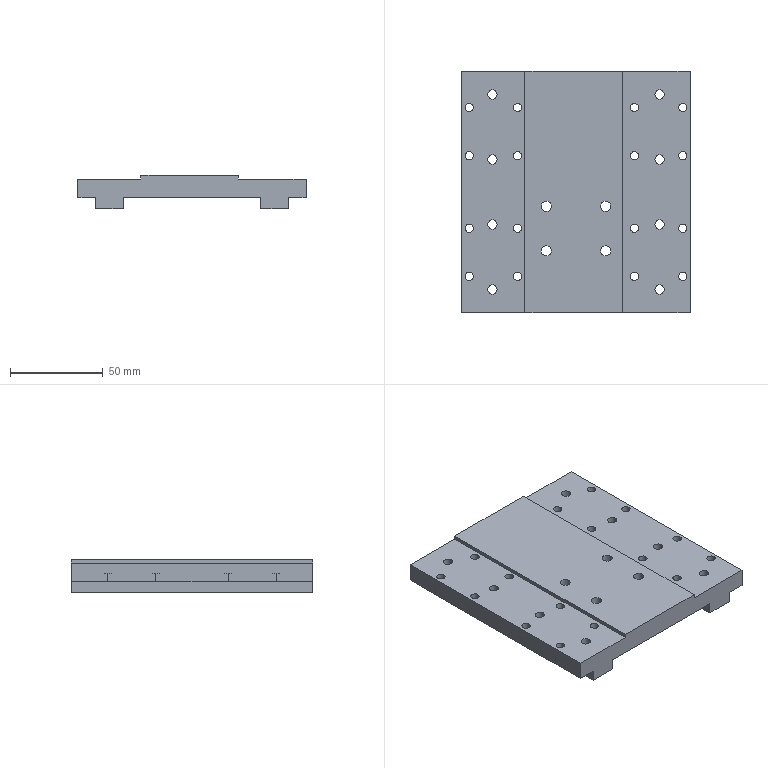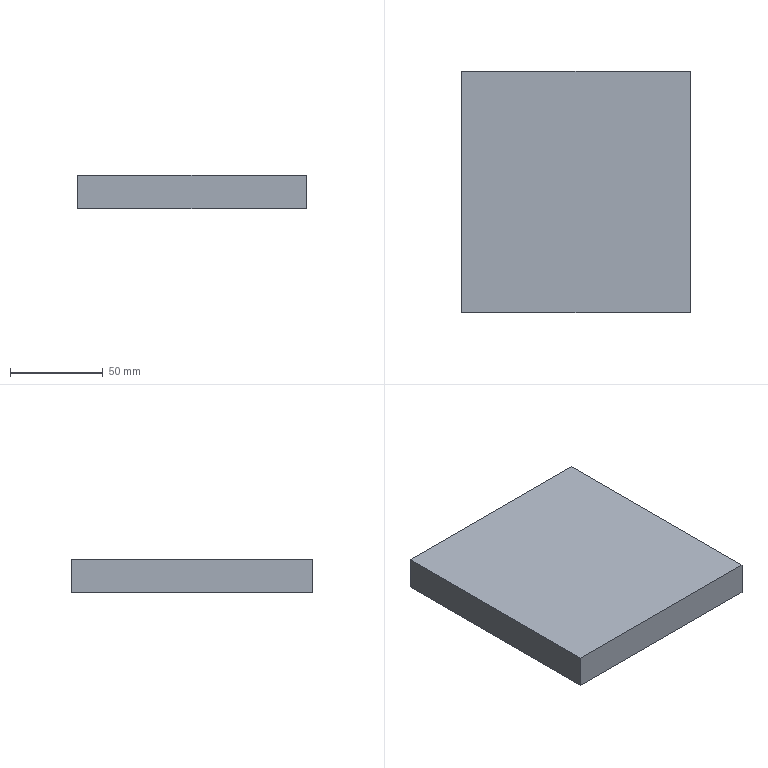CAM job | NX | 3-axis milling, drilling | part box 123 x 130 x 18 mm | stock box 123 x 130 x 18 mm
Tools:
number,name,description,diameter,corner_radius,flute_length,length,flutes
1,D6A45,Milling Tool-5 Parameters,6.0,0.0,50.0,75.0,2
9,5.5ZT,Drilling Tool,5.5,0.0,35.0,50.0,2
16,5.0ZT,Drilling Tool,5.0,0.0,35.0,50.0,2
8,4.5ZT,Drilling Tool,4.5,0.0,35.0,50.0,2
15,D10,Milling Tool-5 Parameters,10.0,0.0,50.0,75.0,2
14,D10JING,Milling Tool-5 Parameters,10.0,0.0,50.0,75.0,2
11,D4,Milling Tool-5 Parameters,4.0,0.0,30.0,30.0,4
12,D6,Milling Tool-5 Parameters,6.0,0.0,50.0,75.0,2
Operations:
program,operation,operation_type,tool,method,geometry_group,spindle_rpm,surface_speed,feed_per_tooth,feed_cut,feed_plunge,cut_length_mm,path_length_mm,cut_time_min,machine_time_min
1,DRILLING,Operation,D6A45,METHOD,A,5000.0,94.0,0.035,350.0,0.0,112.0,874.568,0.32,0.3963
1,DRILLING_COPY_COPY,Operation,5.5ZT,METHOD,A,2000.0,26.0,0.075,300.0,0.0,50.609,250.733,0.1687,0.1887
1,DRILLING_COPY_COPY_COPY,Operation,5.0ZT,METHOD,A,2000.0,26.0,0.075,300.0,0.0,192.017,765.854,0.6401,0.6974
1,DRILLING_COPY_COPY_COPY_COPY,Operation,4.5ZT,METHOD,A,2000.0,26.0,0.075,300.0,0.0,213.631,987.634,0.7121,0.7895
1,ZLEVEL_PROFILE,ZLevelMilling,D10,METHOD,A,9500.0,298.0,0.1579,3000.0,1000.0,10271.268,10345.668,3.455,3.463
1,FLOOR_WALL_1,VolumeBased25DMillingOperation,D10,METHOD,A,9500.0,298.0,0.1579,3000.0,100.0,3275.69,3552.814,1.092,1.12
1,FLOOR_WALL_COPY,VolumeBased25DMillingOperation,D10JING,METHOD,A,9500.0,298.0,0.0789,1500.0,100.0,2470.019,2774.915,1.647,1.677
1,PLANAR_MILL_COPY_COPY_COPY,PlanarMilling,D6A45,METHOD,A,9500.0,179.0,0.0658,1250.0,100.0,442.622,850.17,0.3541,0.3949
1,PLANAR_MILL_COPY_COPY_COPY_COPY,PlanarMilling,D6A45,METHOD,A,9500.0,179.0,0.0658,1250.0,100.0,785.734,3072.632,0.6286,0.8573
1,ZLEVEL_PROFILE_COPY_1,ZLevelMilling,D10JING,METHOD,A,9500.0,298.0,0.0632,1200.0,1000.0,2719.591,2811.891,2.272,2.281
2,FLOOR_WALL_1_COPY,VolumeBased25DMillingOperation,D10,METHOD,B,9500.0,298.0,0.1579,3000.0,100.0,11961.145,12579.431,3.987,4.049
2,FLOOR_WALL_COPY_COPY,VolumeBased25DMillingOperation,D10JING,METHOD,B,9500.0,298.0,0.0789,1500.0,100.0,3205.507,3791.304,2.137,2.196
2,HOLE_MILLING,CylinderMilling,D6,METHOD,B,9500.0,119.0,0.0421,1600.0,100.0,1838.345,3861.398,1.149,1.351
2,HOLE_MILLING_COPY,CylinderMilling,D4,METHOD,B,9500.0,119.0,0.0421,1600.0,100.0,413.362,642.362,0.2584,0.2813
2,PLANAR_MILL_COPY_COPY_COPY_COPY_1,PlanarMilling,D6A45,METHOD,B,9500.0,179.0,0.0658,1250.0,100.0,759.257,1775.603,0.6074,0.709
2,PLANAR_MILL_COPY_COPY_COPY_COPY_1_COPY,PlanarMilling,D6A45,METHOD,B,9500.0,179.0,0.0658,1250.0,100.0,447.425,1929.246,0.3579,0.5061
2,刀补,CylinderMilling,D4,METHOD,B,9500.0,119.0,0.0421,1600.0,100.0,72.308,301.308,0.0452,0.0681